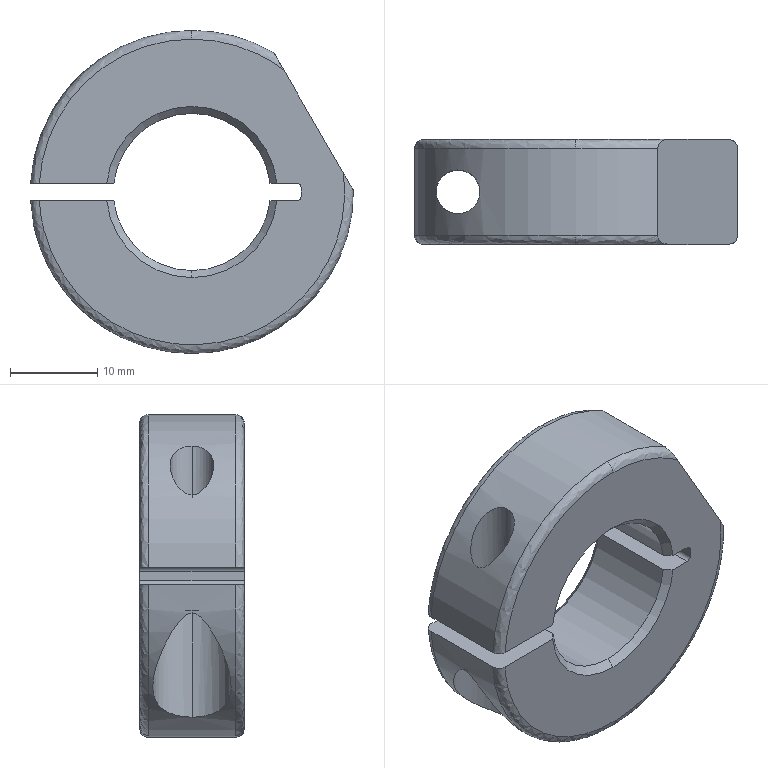Part | STEP file | _X2_95017d2773af_X0_MAB060-14.STEP | 1 solid | 34 faces | box 36.973 x 12 x 37 mm | volume 8292 mm3 | cylinder 14 | plane 9 | spline 6 | cone 5 | commonest cylinder face diameters 18 x3 37 x3 1 x2 5 x2 5.5 x2 9 x2